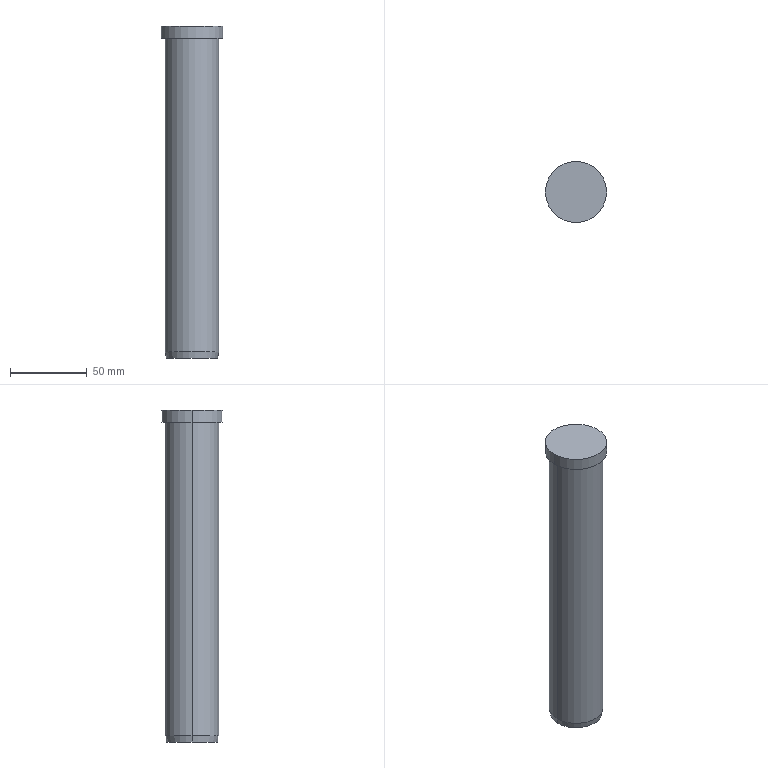Part | Creo | 1 solid | 9 faces | box 40 x 40 x 217 mm | volume 210982 mm3 | cylinder 4 | plane 3 | cone 2 | commonest cylinder face diameters 35 x2 40 x2
STEP:
#1=CARTESIAN_POINT('',(0.,0.,0.));
#2=DIRECTION('',(0.,0.,1.));
#3=DIRECTION('',(1.,0.,0.));
#4=AXIS2_PLACEMENT_3D('',#1,#2,#3);
#5=CARTESIAN_POINT('',(182.,-210.,112.5));
#6=VERTEX_POINT('',#5);
#7=CARTESIAN_POINT('',(142.,-210.,112.5));
#8=VERTEX_POINT('',#7);
#9=CARTESIAN_POINT('',(162.,-210.,112.5));
#10=DIRECTION('',(0.,0.,-1.));
#11=DIRECTION('',(1.,0.,0.));
#12=AXIS2_PLACEMENT_3D('',#9,#10,#11);
#13=CIRCLE('',#12,20.);
#14=EDGE_CURVE('',#6,#8,#13,.T.);
#15=ORIENTED_EDGE('',*,*,#14,.T.);
#16=CARTESIAN_POINT('',(142.,-210.,120.5));
#17=VERTEX_POINT('',#16);
#18=CARTESIAN_POINT('',(142.,-210.,112.5));
#19=DIRECTION('',(0.,0.,1.));
#20=VECTOR('',#19,8.);
#21=LINE('',#18,#20);
#22=EDGE_CURVE('',#8,#17,#21,.T.);
#23=ORIENTED_EDGE('',*,*,#22,.T.);
#24=CARTESIAN_POINT('',(182.,-210.,120.5));
#25=VERTEX_POINT('',#24);
#26=CARTESIAN_POINT('',(162.,-210.,120.5));
#27=DIRECTION('',(0.,0.,1.));
#28=DIRECTION('',(-1.,0.,0.));
#29=AXIS2_PLACEMENT_3D('',#26,#27,#28);
#30=CIRCLE('',#29,20.);
#31=EDGE_CURVE('',#17,#25,#30,.T.);
#32=ORIENTED_EDGE('',*,*,#31,.T.);
#33=CARTESIAN_POINT('',(182.,-210.,112.5));
#34=DIRECTION('',(0.,0.,1.));
#35=VECTOR('',#34,8.);
#36=LINE('',#33,#35);
#37=EDGE_CURVE('',#6,#25,#36,.T.);
#38=ORIENTED_EDGE('',*,*,#37,.F.);
#39=EDGE_LOOP('',(#15,#23,#32,#38));
#40=FACE_OUTER_BOUND('',#39,.F.);
#41=CARTESIAN_POINT('',(162.,-210.,112.5));
#42=DIRECTION('',(0.,0.,1.));
#43=DIRECTION('',(-1.,0.,0.));
#44=AXIS2_PLACEMENT_3D('',#41,#42,#43);
#45=CYLINDRICAL_SURFACE('',#44,20.);
#46=ADVANCED_FACE('',(#40),#45,.T.);
#47=ORIENTED_EDGE('',*,*,#14,.F.);
#48=CARTESIAN_POINT('',(162.,-210.,112.5));
#49=DIRECTION('',(0.,0.,-1.));
#50=DIRECTION('',(-1.,0.,0.));
#51=AXIS2_PLACEMENT_3D('',#48,#49,#50);
#52=CIRCLE('',#51,20.);
#53=EDGE_CURVE('',#8,#6,#52,.T.);
#54=ORIENTED_EDGE('',*,*,#53,.F.);
#55=EDGE_LOOP('',(#47,#54));
#56=FACE_OUTER_BOUND('',#55,.F.);
#57=CARTESIAN_POINT('',(144.5,-210.,112.5));
#58=VERTEX_POINT('',#57);
#59=CARTESIAN_POINT('',(179.5,-210.,112.5));
#60=VERTEX_POINT('',#59);
#61=CARTESIAN_POINT('',(162.,-210.,112.5));
#62=DIRECTION('',(0.,0.,1.));
#63=DIRECTION('',(-1.,0.,0.));
#64=AXIS2_PLACEMENT_3D('',#61,#62,#63);
#65=CIRCLE('',#64,17.5);
#66=EDGE_CURVE('',#58,#60,#65,.T.);
#67=ORIENTED_EDGE('',*,*,#66,.F.);
#68=CARTESIAN_POINT('',(162.,-210.,112.5));
#69=DIRECTION('',(0.,0.,1.));
#70=DIRECTION('',(1.,0.,0.));
#71=AXIS2_PLACEMENT_3D('',#68,#69,#70);
#72=CIRCLE('',#71,17.5);
#73=EDGE_CURVE('',#60,#58,#72,.T.);
#74=ORIENTED_EDGE('',*,*,#73,.F.);
#75=EDGE_LOOP('',(#67,#74));
#76=FACE_BOUND('',#75,.F.);
#77=CARTESIAN_POINT('',(162.,-210.,112.5));
#78=DIRECTION('',(0.,0.,1.));
#79=DIRECTION('',(-1.,0.,0.));
#80=AXIS2_PLACEMENT_3D('',#77,#78,#79);
#81=PLANE('',#80);
#82=ADVANCED_FACE('',(#56,#76),#81,.F.);
#83=CARTESIAN_POINT('',(179.5,-210.,-92.5));
#84=VERTEX_POINT('',#83);
#85=CARTESIAN_POINT('',(144.5,-210.,-92.5));
#86=VERTEX_POINT('',#85);
#87=CARTESIAN_POINT('',(162.,-210.,-92.5));
#88=DIRECTION('',(0.,0.,-1.));
#89=DIRECTION('',(1.,0.,0.));
#90=AXIS2_PLACEMENT_3D('',#87,#88,#89);
#91=CIRCLE('',#90,17.5);
#92=EDGE_CURVE('',#84,#86,#91,.T.);
#93=ORIENTED_EDGE('',*,*,#92,.T.);
#94=CARTESIAN_POINT('',(144.5,-210.,112.5));
#95=DIRECTION('',(0.,0.,-1.));
#96=VECTOR('',#95,205.);
#97=LINE('',#94,#96);
#98=EDGE_CURVE('',#58,#86,#97,.T.);
#99=ORIENTED_EDGE('',*,*,#98,.F.);
#100=ORIENTED_EDGE('',*,*,#66,.T.);
#101=CARTESIAN_POINT('',(179.5,-210.,112.5));
#102=DIRECTION('',(0.,0.,-1.));
#103=VECTOR('',#102,205.);
#104=LINE('',#101,#103);
#105=EDGE_CURVE('',#60,#84,#104,.T.);
#106=ORIENTED_EDGE('',*,*,#105,.T.);
#107=EDGE_LOOP('',(#93,#99,#100,#106));
#108=FACE_OUTER_BOUND('',#107,.F.);
#109=CARTESIAN_POINT('',(162.,-210.,112.5));
#110=DIRECTION('',(0.,0.,-1.));
#111=DIRECTION('',(1.,0.,0.));
#112=AXIS2_PLACEMENT_3D('',#109,#110,#111);
#113=CYLINDRICAL_SURFACE('',#112,17.5);
#114=ADVANCED_FACE('',(#108),#113,.T.);
#115=ORIENTED_EDGE('',*,*,#92,.F.);
#116=CARTESIAN_POINT('',(178.795,-210.,-96.5));
#117=VERTEX_POINT('',#116);
#118=CARTESIAN_POINT('',(178.795,-210.,-96.5));
#119=DIRECTION('',(0.1736,0.,0.9848));
#120=VECTOR('',#119,4.062);
#121=LINE('',#118,#120);
#122=EDGE_CURVE('',#117,#84,#121,.T.);
#123=ORIENTED_EDGE('',*,*,#122,.F.);
#124=CARTESIAN_POINT('',(145.205,-210.,-96.5));
#125=VERTEX_POINT('',#124);
#126=CARTESIAN_POINT('',(162.,-210.,-96.5));
#127=DIRECTION('',(0.,0.,-1.));
#128=DIRECTION('',(1.,0.,0.));
#129=AXIS2_PLACEMENT_3D('',#126,#127,#128);
#130=CIRCLE('',#129,16.795);
#131=EDGE_CURVE('',#117,#125,#130,.T.);
#132=ORIENTED_EDGE('',*,*,#131,.T.);
#133=CARTESIAN_POINT('',(145.205,-210.,-96.5));
#134=DIRECTION('',(-0.1736,0.,0.9848));
#135=VECTOR('',#134,4.062);
#136=LINE('',#133,#135);
#137=EDGE_CURVE('',#125,#86,#136,.T.);
#138=ORIENTED_EDGE('',*,*,#137,.T.);
#139=EDGE_LOOP('',(#115,#123,#132,#138));
#140=FACE_OUTER_BOUND('',#139,.F.);
#141=CARTESIAN_POINT('',(162.,-210.,-94.5));
#142=DIRECTION('',(0.,0.,1.));
#143=DIRECTION('',(-1.,0.,0.));
#144=AXIS2_PLACEMENT_3D('',#141,#142,#143);
#145=CONICAL_SURFACE('',#144,17.147,10.);
#146=ADVANCED_FACE('',(#140),#145,.T.);
#147=CARTESIAN_POINT('',(162.,-210.,-92.5));
#148=DIRECTION('',(0.,0.,-1.));
#149=DIRECTION('',(-1.,0.,0.));
#150=AXIS2_PLACEMENT_3D('',#147,#148,#149);
#151=CIRCLE('',#150,17.5);
#152=EDGE_CURVE('',#86,#84,#151,.T.);
#153=ORIENTED_EDGE('',*,*,#152,.F.);
#154=ORIENTED_EDGE('',*,*,#137,.F.);
#155=CARTESIAN_POINT('',(162.,-210.,-96.5));
#156=DIRECTION('',(0.,0.,-1.));
#157=DIRECTION('',(-1.,0.,0.));
#158=AXIS2_PLACEMENT_3D('',#155,#156,#157);
#159=CIRCLE('',#158,16.795);
#160=EDGE_CURVE('',#125,#117,#159,.T.);
#161=ORIENTED_EDGE('',*,*,#160,.T.);
#162=ORIENTED_EDGE('',*,*,#122,.T.);
#163=EDGE_LOOP('',(#153,#154,#161,#162));
#164=FACE_OUTER_BOUND('',#163,.F.);
#165=CARTESIAN_POINT('',(162.,-210.,-94.5));
#166=DIRECTION('',(0.,0.,1.));
#167=DIRECTION('',(-1.,0.,0.));
#168=AXIS2_PLACEMENT_3D('',#165,#166,#167);
#169=CONICAL_SURFACE('',#168,17.147,10.);
#170=ADVANCED_FACE('',(#164),#169,.T.);
#171=ORIENTED_EDGE('',*,*,#152,.T.);
#172=ORIENTED_EDGE('',*,*,#105,.F.);
#173=ORIENTED_EDGE('',*,*,#73,.T.);
#174=ORIENTED_EDGE('',*,*,#98,.T.);
#175=EDGE_LOOP('',(#171,#172,#173,#174));
#176=FACE_OUTER_BOUND('',#175,.F.);
#177=CARTESIAN_POINT('',(162.,-210.,112.5));
#178=DIRECTION('',(0.,0.,-1.));
#179=DIRECTION('',(1.,0.,0.));
#180=AXIS2_PLACEMENT_3D('',#177,#178,#179);
#181=CYLINDRICAL_SURFACE('',#180,17.5);
#182=ADVANCED_FACE('',(#176),#181,.T.);
#183=ORIENTED_EDGE('',*,*,#160,.F.);
#184=ORIENTED_EDGE('',*,*,#131,.F.);
#185=EDGE_LOOP('',(#183,#184));
#186=FACE_OUTER_BOUND('',#185,.F.);
#187=CARTESIAN_POINT('',(162.,-210.,-96.5));
#188=DIRECTION('',(0.,0.,-1.));
#189=DIRECTION('',(1.,0.,0.));
#190=AXIS2_PLACEMENT_3D('',#187,#188,#189);
#191=PLANE('',#190);
#192=ADVANCED_FACE('',(#186),#191,.T.);
#193=ORIENTED_EDGE('',*,*,#53,.T.);
#194=ORIENTED_EDGE('',*,*,#37,.T.);
#195=CARTESIAN_POINT('',(162.,-210.,120.5));
#196=DIRECTION('',(0.,0.,1.));
#197=DIRECTION('',(1.,0.,0.));
#198=AXIS2_PLACEMENT_3D('',#195,#196,#197);
#199=CIRCLE('',#198,20.);
#200=EDGE_CURVE('',#25,#17,#199,.T.);
#201=ORIENTED_EDGE('',*,*,#200,.T.);
#202=ORIENTED_EDGE('',*,*,#22,.F.);
#203=EDGE_LOOP('',(#193,#194,#201,#202));
#204=FACE_OUTER_BOUND('',#203,.F.);
#205=CARTESIAN_POINT('',(162.,-210.,112.5));
#206=DIRECTION('',(0.,0.,1.));
#207=DIRECTION('',(-1.,0.,0.));
#208=AXIS2_PLACEMENT_3D('',#205,#206,#207);
#209=CYLINDRICAL_SURFACE('',#208,20.);
#210=ADVANCED_FACE('',(#204),#209,.T.);
#211=ORIENTED_EDGE('',*,*,#200,.F.);
#212=ORIENTED_EDGE('',*,*,#31,.F.);
#213=EDGE_LOOP('',(#211,#212));
#214=FACE_OUTER_BOUND('',#213,.F.);
#215=CARTESIAN_POINT('',(162.,-210.,120.5));
#216=DIRECTION('',(0.,0.,1.));
#217=DIRECTION('',(-1.,0.,0.));
#218=AXIS2_PLACEMENT_3D('',#215,#216,#217);
#219=PLANE('',#218);
#220=ADVANCED_FACE('',(#214),#219,.T.);
#221=CLOSED_SHELL('',(#46,#82,#114,#146,#170,#182,#192,#210,#220));
#222=MANIFOLD_SOLID_BREP('',#221);
#223=(LENGTH_UNIT()NAMED_UNIT(*)SI_UNIT(.MILLI.,.METRE.));
#224=UNCERTAINTY_MEASURE_WITH_UNIT(LENGTH_MEASURE(0.02243),#223,'','');
#225=(NAMED_UNIT(*)PLANE_ANGLE_UNIT()SI_UNIT($,.RADIAN.));
#226=PLANE_ANGLE_MEASURE_WITH_UNIT(PLANE_ANGLE_MEASURE(0.01745),#225);
#227=(CONVERSION_BASED_UNIT('DEGREE',#226)NAMED_UNIT(*)PLANE_ANGLE_UNIT());
#228=(NAMED_UNIT(*)SI_UNIT($,.STERADIAN.)SOLID_ANGLE_UNIT());
#229=(GEOMETRIC_REPRESENTATION_CONTEXT(3)GLOBAL_UNCERTAINTY_ASSIGNED_CONTEXT((#224))GLOBAL_UNIT_ASSIGNED_CONTEXT((#223,#227,#228))REPRESENTATION_CONTEXT('',''));
#230=ADVANCED_BREP_SHAPE_REPRESENTATION('',(#4,#222),#229);